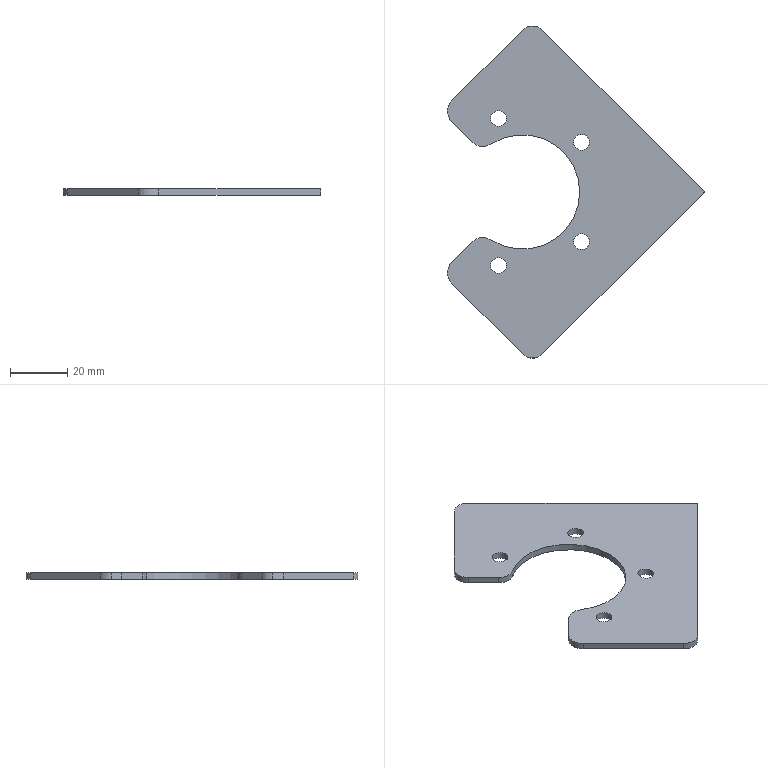Part | SolidWorks | features FlatPattern 1, SMBaseFlange 1, SheetMetal 1 | 1 solid | 25 faces | box 89.853 x 116.066 x 2.3 mm | volume 10484 mm3 | cylinder 17 | plane 8 | commonest cylinder face diameters 5.5 x8 10 x8 40 x1
STEP:
#1=CARTESIAN_POINT('',(-11.093,-25.679,2.3));
#2=VERTEX_POINT('',#1);
#3=CARTESIAN_POINT('',(-5.593,-25.679,2.3));
#4=VERTEX_POINT('',#3);
#5=CARTESIAN_POINT('',(-8.343,-25.679,2.3));
#6=DIRECTION('',(0.,0.,1.));
#7=DIRECTION('',(1.,0.,0.));
#8=AXIS2_PLACEMENT_3D('',#5,#6,#7);
#9=CIRCLE('',#8,2.75);
#10=EDGE_CURVE('',#2,#4,#9,.T.);
#11=ORIENTED_EDGE('',*,*,#10,.T.);
#12=CARTESIAN_POINT('',(-5.593,-25.679,0.));
#13=VERTEX_POINT('',#12);
#14=CARTESIAN_POINT('',(-5.593,-25.679,2.3));
#15=DIRECTION('',(0.,0.,-1.));
#16=VECTOR('',#15,1000.);
#17=LINE('',#14,#16);
#18=EDGE_CURVE('',#4,#13,#17,.T.);
#19=ORIENTED_EDGE('',*,*,#18,.T.);
#20=CARTESIAN_POINT('',(-11.093,-25.679,0.));
#21=VERTEX_POINT('',#20);
#22=CARTESIAN_POINT('',(-8.343,-25.679,0.));
#23=DIRECTION('',(0.,0.,1.));
#24=DIRECTION('',(1.,0.,0.));
#25=AXIS2_PLACEMENT_3D('',#22,#23,#24);
#26=CIRCLE('',#25,2.75);
#27=EDGE_CURVE('',#21,#13,#26,.T.);
#28=ORIENTED_EDGE('',*,*,#27,.F.);
#29=CARTESIAN_POINT('',(-11.093,-25.679,2.3));
#30=DIRECTION('',(0.,0.,-1.));
#31=VECTOR('',#30,1000.);
#32=LINE('',#29,#31);
#33=EDGE_CURVE('',#2,#21,#32,.T.);
#34=ORIENTED_EDGE('',*,*,#33,.F.);
#35=EDGE_LOOP('',(#11,#19,#28,#34));
#36=FACE_OUTER_BOUND('',#35,.T.);
#37=CARTESIAN_POINT('',(-8.343,-25.679,2.3));
#38=DIRECTION('',(0.,0.,-1.));
#39=DIRECTION('',(-1.,0.,0.));
#40=AXIS2_PLACEMENT_3D('',#37,#38,#39);
#41=CYLINDRICAL_SURFACE('',#40,2.75);
#42=ADVANCED_FACE('',(#36),#41,.F.);
#43=CARTESIAN_POINT('',(-11.093,25.679,2.3));
#44=VERTEX_POINT('',#43);
#45=CARTESIAN_POINT('',(-5.593,25.679,2.3));
#46=VERTEX_POINT('',#45);
#47=CARTESIAN_POINT('',(-8.343,25.679,2.3));
#48=DIRECTION('',(0.,0.,1.));
#49=DIRECTION('',(1.,0.,0.));
#50=AXIS2_PLACEMENT_3D('',#47,#48,#49);
#51=CIRCLE('',#50,2.75);
#52=EDGE_CURVE('',#44,#46,#51,.T.);
#53=ORIENTED_EDGE('',*,*,#52,.T.);
#54=CARTESIAN_POINT('',(-5.593,25.679,0.));
#55=VERTEX_POINT('',#54);
#56=CARTESIAN_POINT('',(-5.593,25.679,2.3));
#57=DIRECTION('',(0.,0.,-1.));
#58=VECTOR('',#57,1000.);
#59=LINE('',#56,#58);
#60=EDGE_CURVE('',#46,#55,#59,.T.);
#61=ORIENTED_EDGE('',*,*,#60,.T.);
#62=CARTESIAN_POINT('',(-11.093,25.679,0.));
#63=VERTEX_POINT('',#62);
#64=CARTESIAN_POINT('',(-8.343,25.679,0.));
#65=DIRECTION('',(0.,0.,1.));
#66=DIRECTION('',(1.,0.,0.));
#67=AXIS2_PLACEMENT_3D('',#64,#65,#66);
#68=CIRCLE('',#67,2.75);
#69=EDGE_CURVE('',#63,#55,#68,.T.);
#70=ORIENTED_EDGE('',*,*,#69,.F.);
#71=CARTESIAN_POINT('',(-11.093,25.679,2.3));
#72=DIRECTION('',(0.,0.,-1.));
#73=VECTOR('',#72,1000.);
#74=LINE('',#71,#73);
#75=EDGE_CURVE('',#44,#63,#74,.T.);
#76=ORIENTED_EDGE('',*,*,#75,.F.);
#77=EDGE_LOOP('',(#53,#61,#70,#76));
#78=FACE_OUTER_BOUND('',#77,.T.);
#79=CARTESIAN_POINT('',(-8.343,25.679,2.3));
#80=DIRECTION('',(0.,0.,-1.));
#81=DIRECTION('',(-1.,0.,0.));
#82=AXIS2_PLACEMENT_3D('',#79,#80,#81);
#83=CYLINDRICAL_SURFACE('',#82,2.75);
#84=ADVANCED_FACE('',(#78),#83,.F.);
#85=CARTESIAN_POINT('',(17.933,17.355,2.3));
#86=VERTEX_POINT('',#85);
#87=CARTESIAN_POINT('',(23.433,17.355,2.3));
#88=VERTEX_POINT('',#87);
#89=CARTESIAN_POINT('',(20.683,17.355,2.3));
#90=DIRECTION('',(0.,0.,1.));
#91=DIRECTION('',(1.,0.,0.));
#92=AXIS2_PLACEMENT_3D('',#89,#90,#91);
#93=CIRCLE('',#92,2.75);
#94=EDGE_CURVE('',#86,#88,#93,.T.);
#95=ORIENTED_EDGE('',*,*,#94,.T.);
#96=CARTESIAN_POINT('',(23.433,17.355,0.));
#97=VERTEX_POINT('',#96);
#98=CARTESIAN_POINT('',(23.433,17.355,2.3));
#99=DIRECTION('',(0.,0.,-1.));
#100=VECTOR('',#99,1000.);
#101=LINE('',#98,#100);
#102=EDGE_CURVE('',#88,#97,#101,.T.);
#103=ORIENTED_EDGE('',*,*,#102,.T.);
#104=CARTESIAN_POINT('',(17.933,17.355,0.));
#105=VERTEX_POINT('',#104);
#106=CARTESIAN_POINT('',(20.683,17.355,0.));
#107=DIRECTION('',(0.,0.,1.));
#108=DIRECTION('',(1.,0.,0.));
#109=AXIS2_PLACEMENT_3D('',#106,#107,#108);
#110=CIRCLE('',#109,2.75);
#111=EDGE_CURVE('',#105,#97,#110,.T.);
#112=ORIENTED_EDGE('',*,*,#111,.F.);
#113=CARTESIAN_POINT('',(17.933,17.355,2.3));
#114=DIRECTION('',(0.,0.,-1.));
#115=VECTOR('',#114,1000.);
#116=LINE('',#113,#115);
#117=EDGE_CURVE('',#86,#105,#116,.T.);
#118=ORIENTED_EDGE('',*,*,#117,.F.);
#119=EDGE_LOOP('',(#95,#103,#112,#118));
#120=FACE_OUTER_BOUND('',#119,.T.);
#121=CARTESIAN_POINT('',(20.683,17.355,2.3));
#122=DIRECTION('',(0.,0.,-1.));
#123=DIRECTION('',(-1.,0.,0.));
#124=AXIS2_PLACEMENT_3D('',#121,#122,#123);
#125=CYLINDRICAL_SURFACE('',#124,2.75);
#126=ADVANCED_FACE('',(#120),#125,.F.);
#127=CARTESIAN_POINT('',(17.933,-17.355,2.3));
#128=VERTEX_POINT('',#127);
#129=CARTESIAN_POINT('',(23.433,-17.355,2.3));
#130=VERTEX_POINT('',#129);
#131=CARTESIAN_POINT('',(20.683,-17.355,2.3));
#132=DIRECTION('',(0.,0.,1.));
#133=DIRECTION('',(1.,0.,0.));
#134=AXIS2_PLACEMENT_3D('',#131,#132,#133);
#135=CIRCLE('',#134,2.75);
#136=EDGE_CURVE('',#128,#130,#135,.T.);
#137=ORIENTED_EDGE('',*,*,#136,.T.);
#138=CARTESIAN_POINT('',(23.433,-17.355,0.));
#139=VERTEX_POINT('',#138);
#140=CARTESIAN_POINT('',(23.433,-17.355,2.3));
#141=DIRECTION('',(0.,0.,-1.));
#142=VECTOR('',#141,1000.);
#143=LINE('',#140,#142);
#144=EDGE_CURVE('',#130,#139,#143,.T.);
#145=ORIENTED_EDGE('',*,*,#144,.T.);
#146=CARTESIAN_POINT('',(17.933,-17.355,0.));
#147=VERTEX_POINT('',#146);
#148=CARTESIAN_POINT('',(20.683,-17.355,0.));
#149=DIRECTION('',(0.,0.,1.));
#150=DIRECTION('',(1.,0.,0.));
#151=AXIS2_PLACEMENT_3D('',#148,#149,#150);
#152=CIRCLE('',#151,2.75);
#153=EDGE_CURVE('',#147,#139,#152,.T.);
#154=ORIENTED_EDGE('',*,*,#153,.F.);
#155=CARTESIAN_POINT('',(17.933,-17.355,2.3));
#156=DIRECTION('',(0.,0.,-1.));
#157=VECTOR('',#156,1000.);
#158=LINE('',#155,#157);
#159=EDGE_CURVE('',#128,#147,#158,.T.);
#160=ORIENTED_EDGE('',*,*,#159,.F.);
#161=EDGE_LOOP('',(#137,#145,#154,#160));
#162=FACE_OUTER_BOUND('',#161,.T.);
#163=CARTESIAN_POINT('',(20.683,-17.355,2.3));
#164=DIRECTION('',(0.,0.,-1.));
#165=DIRECTION('',(-1.,0.,0.));
#166=AXIS2_PLACEMENT_3D('',#163,#164,#165);
#167=CYLINDRICAL_SURFACE('',#166,2.75);
#168=ADVANCED_FACE('',(#162),#167,.F.);
#169=CARTESIAN_POINT('',(-26.213,-28.284,2.3));
#170=VERTEX_POINT('',#169);
#171=CARTESIAN_POINT('',(-24.749,-31.82,2.3));
#172=VERTEX_POINT('',#171);
#173=CARTESIAN_POINT('',(-21.213,-28.284,2.3));
#174=DIRECTION('',(0.,0.,1.));
#175=DIRECTION('',(-1.,0.,0.));
#176=AXIS2_PLACEMENT_3D('',#173,#174,#175);
#177=CIRCLE('',#176,5.);
#178=EDGE_CURVE('',#170,#172,#177,.T.);
#179=ORIENTED_EDGE('',*,*,#178,.F.);
#180=CARTESIAN_POINT('',(-26.213,-28.284,0.));
#181=VERTEX_POINT('',#180);
#182=CARTESIAN_POINT('',(-26.213,-28.284,2.3));
#183=DIRECTION('',(0.,0.,-1.));
#184=VECTOR('',#183,1000.);
#185=LINE('',#182,#184);
#186=EDGE_CURVE('',#170,#181,#185,.T.);
#187=ORIENTED_EDGE('',*,*,#186,.T.);
#188=CARTESIAN_POINT('',(-24.749,-31.82,0.));
#189=VERTEX_POINT('',#188);
#190=CARTESIAN_POINT('',(-21.213,-28.284,0.));
#191=DIRECTION('',(0.,0.,1.));
#192=DIRECTION('',(-1.,0.,0.));
#193=AXIS2_PLACEMENT_3D('',#190,#191,#192);
#194=CIRCLE('',#193,5.);
#195=EDGE_CURVE('',#181,#189,#194,.T.);
#196=ORIENTED_EDGE('',*,*,#195,.T.);
#197=CARTESIAN_POINT('',(-24.749,-31.82,2.3));
#198=DIRECTION('',(0.,0.,-1.));
#199=VECTOR('',#198,1000.);
#200=LINE('',#197,#199);
#201=EDGE_CURVE('',#172,#189,#200,.T.);
#202=ORIENTED_EDGE('',*,*,#201,.F.);
#203=EDGE_LOOP('',(#179,#187,#196,#202));
#204=FACE_OUTER_BOUND('',#203,.T.);
#205=CARTESIAN_POINT('',(-21.213,-28.284,2.3));
#206=DIRECTION('',(0.,0.,-1.));
#207=DIRECTION('',(-1.,0.,0.));
#208=AXIS2_PLACEMENT_3D('',#205,#206,#207);
#209=CYLINDRICAL_SURFACE('',#208,5.);
#210=ADVANCED_FACE('',(#204),#209,.T.);
#211=CARTESIAN_POINT('',(-26.213,28.284,2.3));
#212=VERTEX_POINT('',#211);
#213=CARTESIAN_POINT('',(-24.749,24.749,2.3));
#214=VERTEX_POINT('',#213);
#215=CARTESIAN_POINT('',(-21.213,28.284,2.3));
#216=DIRECTION('',(0.,0.,1.));
#217=DIRECTION('',(-1.,0.,0.));
#218=AXIS2_PLACEMENT_3D('',#215,#216,#217);
#219=CIRCLE('',#218,5.);
#220=EDGE_CURVE('',#212,#214,#219,.T.);
#221=ORIENTED_EDGE('',*,*,#220,.F.);
#222=CARTESIAN_POINT('',(-26.213,28.284,0.));
#223=VERTEX_POINT('',#222);
#224=CARTESIAN_POINT('',(-26.213,28.284,2.3));
#225=DIRECTION('',(0.,0.,-1.));
#226=VECTOR('',#225,1000.);
#227=LINE('',#224,#226);
#228=EDGE_CURVE('',#212,#223,#227,.T.);
#229=ORIENTED_EDGE('',*,*,#228,.T.);
#230=CARTESIAN_POINT('',(-24.749,24.749,0.));
#231=VERTEX_POINT('',#230);
#232=CARTESIAN_POINT('',(-21.213,28.284,0.));
#233=DIRECTION('',(0.,0.,1.));
#234=DIRECTION('',(-1.,0.,0.));
#235=AXIS2_PLACEMENT_3D('',#232,#233,#234);
#236=CIRCLE('',#235,5.);
#237=EDGE_CURVE('',#223,#231,#236,.T.);
#238=ORIENTED_EDGE('',*,*,#237,.T.);
#239=CARTESIAN_POINT('',(-24.749,24.749,2.3));
#240=DIRECTION('',(0.,0.,-1.));
#241=VECTOR('',#240,1000.);
#242=LINE('',#239,#241);
#243=EDGE_CURVE('',#214,#231,#242,.T.);
#244=ORIENTED_EDGE('',*,*,#243,.F.);
#245=EDGE_LOOP('',(#221,#229,#238,#244));
#246=FACE_OUTER_BOUND('',#245,.T.);
#247=CARTESIAN_POINT('',(-21.213,28.284,2.3));
#248=DIRECTION('',(0.,0.,-1.));
#249=DIRECTION('',(-1.,0.,0.));
#250=AXIS2_PLACEMENT_3D('',#247,#248,#249);
#251=CYLINDRICAL_SURFACE('',#250,5.);
#252=ADVANCED_FACE('',(#246),#251,.T.);
#253=CARTESIAN_POINT('',(-24.749,31.82,2.3));
#254=VERTEX_POINT('',#253);
#255=CARTESIAN_POINT('',(-21.213,28.284,2.3));
#256=DIRECTION('',(0.,0.,1.));
#257=DIRECTION('',(-1.,0.,0.));
#258=AXIS2_PLACEMENT_3D('',#255,#256,#257);
#259=CIRCLE('',#258,5.);
#260=EDGE_CURVE('',#254,#212,#259,.T.);
#261=ORIENTED_EDGE('',*,*,#260,.T.);
#262=ORIENTED_EDGE('',*,*,#220,.T.);
#263=CARTESIAN_POINT('',(-17.321,17.321,2.3));
#264=VERTEX_POINT('',#263);
#265=CARTESIAN_POINT('',(-17.321,17.321,2.3));
#266=DIRECTION('',(0.7071,-0.7071,0.));
#267=VECTOR('',#266,1000.);
#268=LINE('',#265,#267);
#269=EDGE_CURVE('',#214,#264,#268,.T.);
#270=ORIENTED_EDGE('',*,*,#269,.T.);
#271=CARTESIAN_POINT('',(-11.028,16.685,2.3));
#272=VERTEX_POINT('',#271);
#273=CARTESIAN_POINT('',(-13.785,20.856,2.3));
#274=DIRECTION('',(0.,0.,1.));
#275=DIRECTION('',(1.,0.,0.));
#276=AXIS2_PLACEMENT_3D('',#273,#274,#275);
#277=CIRCLE('',#276,5.);
#278=EDGE_CURVE('',#264,#272,#277,.T.);
#279=ORIENTED_EDGE('',*,*,#278,.T.);
#280=CARTESIAN_POINT('',(-11.028,-16.685,2.3));
#281=VERTEX_POINT('',#280);
#282=CARTESIAN_POINT('',(0.,0.,2.3));
#283=DIRECTION('',(0.,0.,-1.));
#284=DIRECTION('',(1.,0.,0.));
#285=AXIS2_PLACEMENT_3D('',#282,#283,#284);
#286=CIRCLE('',#285,20.);
#287=EDGE_CURVE('',#272,#281,#286,.T.);
#288=ORIENTED_EDGE('',*,*,#287,.T.);
#289=CARTESIAN_POINT('',(-17.321,-17.321,2.3));
#290=VERTEX_POINT('',#289);
#291=CARTESIAN_POINT('',(-13.785,-20.856,2.3));
#292=DIRECTION('',(0.,0.,1.));
#293=DIRECTION('',(-1.,0.,0.));
#294=AXIS2_PLACEMENT_3D('',#291,#292,#293);
#295=CIRCLE('',#294,5.);
#296=EDGE_CURVE('',#281,#290,#295,.T.);
#297=ORIENTED_EDGE('',*,*,#296,.T.);
#298=CARTESIAN_POINT('',(-24.749,-24.749,2.3));
#299=VERTEX_POINT('',#298);
#300=CARTESIAN_POINT('',(-24.749,-24.749,2.3));
#301=DIRECTION('',(-0.7071,-0.7071,0.));
#302=VECTOR('',#301,1000.);
#303=LINE('',#300,#302);
#304=EDGE_CURVE('',#290,#299,#303,.T.);
#305=ORIENTED_EDGE('',*,*,#304,.T.);
#306=CARTESIAN_POINT('',(-21.213,-28.284,2.3));
#307=DIRECTION('',(0.,0.,1.));
#308=DIRECTION('',(-1.,0.,0.));
#309=AXIS2_PLACEMENT_3D('',#306,#307,#308);
#310=CIRCLE('',#309,5.);
#311=EDGE_CURVE('',#299,#170,#310,.T.);
#312=ORIENTED_EDGE('',*,*,#311,.T.);
#313=ORIENTED_EDGE('',*,*,#178,.T.);
#314=CARTESIAN_POINT('',(0.00006304,-56.568,2.3));
#315=VERTEX_POINT('',#314);
#316=CARTESIAN_POINT('',(0.00006304,-56.568,2.3));
#317=DIRECTION('',(0.7071,-0.7071,0.));
#318=VECTOR('',#317,1000.);
#319=LINE('',#316,#318);
#320=EDGE_CURVE('',#172,#315,#319,.T.);
#321=ORIENTED_EDGE('',*,*,#320,.T.);
#322=CARTESIAN_POINT('',(7.071,-56.568,2.3));
#323=VERTEX_POINT('',#322);
#324=CARTESIAN_POINT('',(3.536,-53.033,2.3));
#325=DIRECTION('',(0.,0.,1.));
#326=DIRECTION('',(1.,0.,0.));
#327=AXIS2_PLACEMENT_3D('',#324,#325,#326);
#328=CIRCLE('',#327,5.);
#329=EDGE_CURVE('',#315,#323,#328,.T.);
#330=ORIENTED_EDGE('',*,*,#329,.T.);
#331=CARTESIAN_POINT('',(63.64,0.00006304,2.3));
#332=VERTEX_POINT('',#331);
#333=CARTESIAN_POINT('',(7.071,-56.568,2.3));
#334=DIRECTION('',(0.7071,0.7071,0.));
#335=VECTOR('',#334,1000.);
#336=LINE('',#333,#335);
#337=EDGE_CURVE('',#323,#332,#336,.T.);
#338=ORIENTED_EDGE('',*,*,#337,.T.);
#339=CARTESIAN_POINT('',(7.071,56.569,2.3));
#340=VERTEX_POINT('',#339);
#341=CARTESIAN_POINT('',(7.071,56.569,2.3));
#342=DIRECTION('',(-0.7071,0.7071,0.));
#343=VECTOR('',#342,1000.);
#344=LINE('',#341,#343);
#345=EDGE_CURVE('',#332,#340,#344,.T.);
#346=ORIENTED_EDGE('',*,*,#345,.T.);
#347=CARTESIAN_POINT('',(0.000003708,56.569,2.3));
#348=VERTEX_POINT('',#347);
#349=CARTESIAN_POINT('',(3.536,53.033,2.3));
#350=DIRECTION('',(0.,0.,1.));
#351=DIRECTION('',(-1.,0.,0.));
#352=AXIS2_PLACEMENT_3D('',#349,#350,#351);
#353=CIRCLE('',#352,5.);
#354=EDGE_CURVE('',#340,#348,#353,.T.);
#355=ORIENTED_EDGE('',*,*,#354,.T.);
#356=CARTESIAN_POINT('',(-24.749,31.82,2.3));
#357=DIRECTION('',(-0.7071,-0.7071,0.));
#358=VECTOR('',#357,1000.);
#359=LINE('',#356,#358);
#360=EDGE_CURVE('',#348,#254,#359,.T.);
#361=ORIENTED_EDGE('',*,*,#360,.T.);
#362=EDGE_LOOP('',(#261,#262,#270,#279,#288,#297,#305,#312,#313,#321,#330,#338,#346,#355,#361));
#363=FACE_OUTER_BOUND('',#362,.T.);
#364=ORIENTED_EDGE('',*,*,#136,.F.);
#365=CARTESIAN_POINT('',(20.683,-17.355,2.3));
#366=DIRECTION('',(0.,0.,1.));
#367=DIRECTION('',(1.,0.,0.));
#368=AXIS2_PLACEMENT_3D('',#365,#366,#367);
#369=CIRCLE('',#368,2.75);
#370=EDGE_CURVE('',#130,#128,#369,.T.);
#371=ORIENTED_EDGE('',*,*,#370,.F.);
#372=EDGE_LOOP('',(#364,#371));
#373=FACE_BOUND('',#372,.T.);
#374=ORIENTED_EDGE('',*,*,#94,.F.);
#375=CARTESIAN_POINT('',(20.683,17.355,2.3));
#376=DIRECTION('',(0.,0.,1.));
#377=DIRECTION('',(1.,0.,0.));
#378=AXIS2_PLACEMENT_3D('',#375,#376,#377);
#379=CIRCLE('',#378,2.75);
#380=EDGE_CURVE('',#88,#86,#379,.T.);
#381=ORIENTED_EDGE('',*,*,#380,.F.);
#382=EDGE_LOOP('',(#374,#381));
#383=FACE_BOUND('',#382,.T.);
#384=ORIENTED_EDGE('',*,*,#52,.F.);
#385=CARTESIAN_POINT('',(-8.343,25.679,2.3));
#386=DIRECTION('',(0.,0.,1.));
#387=DIRECTION('',(1.,0.,0.));
#388=AXIS2_PLACEMENT_3D('',#385,#386,#387);
#389=CIRCLE('',#388,2.75);
#390=EDGE_CURVE('',#46,#44,#389,.T.);
#391=ORIENTED_EDGE('',*,*,#390,.F.);
#392=EDGE_LOOP('',(#384,#391));
#393=FACE_BOUND('',#392,.T.);
#394=ORIENTED_EDGE('',*,*,#10,.F.);
#395=CARTESIAN_POINT('',(-8.343,-25.679,2.3));
#396=DIRECTION('',(0.,0.,1.));
#397=DIRECTION('',(1.,0.,0.));
#398=AXIS2_PLACEMENT_3D('',#395,#396,#397);
#399=CIRCLE('',#398,2.75);
#400=EDGE_CURVE('',#4,#2,#399,.T.);
#401=ORIENTED_EDGE('',*,*,#400,.F.);
#402=EDGE_LOOP('',(#394,#401));
#403=FACE_BOUND('',#402,.T.);
#404=CARTESIAN_POINT('',(-21.213,28.284,2.3));
#405=DIRECTION('',(0.,0.,-1.));
#406=DIRECTION('',(-1.,0.,0.));
#407=AXIS2_PLACEMENT_3D('',#404,#405,#406);
#408=PLANE('',#407);
#409=ADVANCED_FACE('',(#363,#373,#383,#393,#403),#408,.F.);
#410=ORIENTED_EDGE('',*,*,#69,.T.);
#411=CARTESIAN_POINT('',(-8.343,25.679,0.));
#412=DIRECTION('',(0.,0.,1.));
#413=DIRECTION('',(1.,0.,0.));
#414=AXIS2_PLACEMENT_3D('',#411,#412,#413);
#415=CIRCLE('',#414,2.75);
#416=EDGE_CURVE('',#55,#63,#415,.T.);
#417=ORIENTED_EDGE('',*,*,#416,.T.);
#418=EDGE_LOOP('',(#410,#417));
#419=FACE_BOUND('',#418,.T.);
#420=ORIENTED_EDGE('',*,*,#153,.T.);
#421=CARTESIAN_POINT('',(20.683,-17.355,0.));
#422=DIRECTION('',(0.,0.,1.));
#423=DIRECTION('',(1.,0.,0.));
#424=AXIS2_PLACEMENT_3D('',#421,#422,#423);
#425=CIRCLE('',#424,2.75);
#426=EDGE_CURVE('',#139,#147,#425,.T.);
#427=ORIENTED_EDGE('',*,*,#426,.T.);
#428=EDGE_LOOP('',(#420,#427));
#429=FACE_BOUND('',#428,.T.);
#430=CARTESIAN_POINT('',(-24.749,31.82,0.));
#431=VERTEX_POINT('',#430);
#432=CARTESIAN_POINT('',(-21.213,28.284,0.));
#433=DIRECTION('',(0.,0.,1.));
#434=DIRECTION('',(-1.,0.,0.));
#435=AXIS2_PLACEMENT_3D('',#432,#433,#434);
#436=CIRCLE('',#435,5.);
#437=EDGE_CURVE('',#431,#223,#436,.T.);
#438=ORIENTED_EDGE('',*,*,#437,.F.);
#439=CARTESIAN_POINT('',(0.000003708,56.569,0.));
#440=VERTEX_POINT('',#439);
#441=CARTESIAN_POINT('',(-24.749,31.82,0.));
#442=DIRECTION('',(-0.7071,-0.7071,0.));
#443=VECTOR('',#442,1000.);
#444=LINE('',#441,#443);
#445=EDGE_CURVE('',#440,#431,#444,.T.);
#446=ORIENTED_EDGE('',*,*,#445,.F.);
#447=CARTESIAN_POINT('',(7.071,56.569,0.));
#448=VERTEX_POINT('',#447);
#449=CARTESIAN_POINT('',(3.536,53.033,0.));
#450=DIRECTION('',(0.,0.,1.));
#451=DIRECTION('',(-1.,0.,0.));
#452=AXIS2_PLACEMENT_3D('',#449,#450,#451);
#453=CIRCLE('',#452,5.);
#454=EDGE_CURVE('',#448,#440,#453,.T.);
#455=ORIENTED_EDGE('',*,*,#454,.F.);
#456=CARTESIAN_POINT('',(63.64,0.00006304,0.));
#457=VERTEX_POINT('',#456);
#458=CARTESIAN_POINT('',(7.071,56.569,0.));
#459=DIRECTION('',(-0.7071,0.7071,0.));
#460=VECTOR('',#459,1000.);
#461=LINE('',#458,#460);
#462=EDGE_CURVE('',#457,#448,#461,.T.);
#463=ORIENTED_EDGE('',*,*,#462,.F.);
#464=CARTESIAN_POINT('',(7.071,-56.568,0.));
#465=VERTEX_POINT('',#464);
#466=CARTESIAN_POINT('',(7.071,-56.568,0.));
#467=DIRECTION('',(0.7071,0.7071,0.));
#468=VECTOR('',#467,1000.);
#469=LINE('',#466,#468);
#470=EDGE_CURVE('',#465,#457,#469,.T.);
#471=ORIENTED_EDGE('',*,*,#470,.F.);
#472=CARTESIAN_POINT('',(0.00006304,-56.568,0.));
#473=VERTEX_POINT('',#472);
#474=CARTESIAN_POINT('',(3.536,-53.033,0.));
#475=DIRECTION('',(0.,0.,1.));
#476=DIRECTION('',(1.,0.,0.));
#477=AXIS2_PLACEMENT_3D('',#474,#475,#476);
#478=CIRCLE('',#477,5.);
#479=EDGE_CURVE('',#473,#465,#478,.T.);
#480=ORIENTED_EDGE('',*,*,#479,.F.);
#481=CARTESIAN_POINT('',(0.00006304,-56.568,0.));
#482=DIRECTION('',(0.7071,-0.7071,0.));
#483=VECTOR('',#482,1000.);
#484=LINE('',#481,#483);
#485=EDGE_CURVE('',#189,#473,#484,.T.);
#486=ORIENTED_EDGE('',*,*,#485,.F.);
#487=ORIENTED_EDGE('',*,*,#195,.F.);
#488=CARTESIAN_POINT('',(-24.749,-24.749,0.));
#489=VERTEX_POINT('',#488);
#490=CARTESIAN_POINT('',(-21.213,-28.284,0.));
#491=DIRECTION('',(0.,0.,1.));
#492=DIRECTION('',(-1.,0.,0.));
#493=AXIS2_PLACEMENT_3D('',#490,#491,#492);
#494=CIRCLE('',#493,5.);
#495=EDGE_CURVE('',#489,#181,#494,.T.);
#496=ORIENTED_EDGE('',*,*,#495,.F.);
#497=CARTESIAN_POINT('',(-17.321,-17.321,0.));
#498=VERTEX_POINT('',#497);
#499=CARTESIAN_POINT('',(-24.749,-24.749,0.));
#500=DIRECTION('',(-0.7071,-0.7071,0.));
#501=VECTOR('',#500,1000.);
#502=LINE('',#499,#501);
#503=EDGE_CURVE('',#498,#489,#502,.T.);
#504=ORIENTED_EDGE('',*,*,#503,.F.);
#505=CARTESIAN_POINT('',(-11.028,-16.685,0.));
#506=VERTEX_POINT('',#505);
#507=CARTESIAN_POINT('',(-13.785,-20.856,0.));
#508=DIRECTION('',(0.,0.,1.));
#509=DIRECTION('',(-1.,0.,0.));
#510=AXIS2_PLACEMENT_3D('',#507,#508,#509);
#511=CIRCLE('',#510,5.);
#512=EDGE_CURVE('',#506,#498,#511,.T.);
#513=ORIENTED_EDGE('',*,*,#512,.F.);
#514=CARTESIAN_POINT('',(-11.028,16.685,0.));
#515=VERTEX_POINT('',#514);
#516=CARTESIAN_POINT('',(0.,0.,0.));
#517=DIRECTION('',(0.,0.,-1.));
#518=DIRECTION('',(1.,0.,0.));
#519=AXIS2_PLACEMENT_3D('',#516,#517,#518);
#520=CIRCLE('',#519,20.);
#521=EDGE_CURVE('',#515,#506,#520,.T.);
#522=ORIENTED_EDGE('',*,*,#521,.F.);
#523=CARTESIAN_POINT('',(-17.321,17.321,0.));
#524=VERTEX_POINT('',#523);
#525=CARTESIAN_POINT('',(-13.785,20.856,0.));
#526=DIRECTION('',(0.,0.,1.));
#527=DIRECTION('',(1.,0.,0.));
#528=AXIS2_PLACEMENT_3D('',#525,#526,#527);
#529=CIRCLE('',#528,5.);
#530=EDGE_CURVE('',#524,#515,#529,.T.);
#531=ORIENTED_EDGE('',*,*,#530,.F.);
#532=CARTESIAN_POINT('',(-17.321,17.321,0.));
#533=DIRECTION('',(0.7071,-0.7071,0.));
#534=VECTOR('',#533,1000.);
#535=LINE('',#532,#534);
#536=EDGE_CURVE('',#231,#524,#535,.T.);
#537=ORIENTED_EDGE('',*,*,#536,.F.);
#538=ORIENTED_EDGE('',*,*,#237,.F.);
#539=EDGE_LOOP('',(#438,#446,#455,#463,#471,#480,#486,#487,#496,#504,#513,#522,#531,#537,#538));
#540=FACE_OUTER_BOUND('',#539,.T.);
#541=ORIENTED_EDGE('',*,*,#111,.T.);
#542=CARTESIAN_POINT('',(20.683,17.355,0.));
#543=DIRECTION('',(0.,0.,1.));
#544=DIRECTION('',(1.,0.,0.));
#545=AXIS2_PLACEMENT_3D('',#542,#543,#544);
#546=CIRCLE('',#545,2.75);
#547=EDGE_CURVE('',#97,#105,#546,.T.);
#548=ORIENTED_EDGE('',*,*,#547,.T.);
#549=EDGE_LOOP('',(#541,#548));
#550=FACE_BOUND('',#549,.T.);
#551=ORIENTED_EDGE('',*,*,#27,.T.);
#552=CARTESIAN_POINT('',(-8.343,-25.679,0.));
#553=DIRECTION('',(0.,0.,1.));
#554=DIRECTION('',(1.,0.,0.));
#555=AXIS2_PLACEMENT_3D('',#552,#553,#554);
#556=CIRCLE('',#555,2.75);
#557=EDGE_CURVE('',#13,#21,#556,.T.);
#558=ORIENTED_EDGE('',*,*,#557,.T.);
#559=EDGE_LOOP('',(#551,#558));
#560=FACE_BOUND('',#559,.T.);
#561=CARTESIAN_POINT('',(-21.213,28.284,0.));
#562=DIRECTION('',(0.,0.,-1.));
#563=DIRECTION('',(-1.,0.,0.));
#564=AXIS2_PLACEMENT_3D('',#561,#562,#563);
#565=PLANE('',#564);
#566=ADVANCED_FACE('',(#419,#429,#540,#550,#560),#565,.T.);
#567=ORIENTED_EDGE('',*,*,#228,.F.);
#568=ORIENTED_EDGE('',*,*,#260,.F.);
#569=CARTESIAN_POINT('',(-24.749,31.82,2.3));
#570=DIRECTION('',(0.,0.,-1.));
#571=VECTOR('',#570,1000.);
#572=LINE('',#569,#571);
#573=EDGE_CURVE('',#254,#431,#572,.T.);
#574=ORIENTED_EDGE('',*,*,#573,.T.);
#575=ORIENTED_EDGE('',*,*,#437,.T.);
#576=EDGE_LOOP('',(#567,#568,#574,#575));
#577=FACE_OUTER_BOUND('',#576,.T.);
#578=CARTESIAN_POINT('',(-21.213,28.284,2.3));
#579=DIRECTION('',(0.,0.,-1.));
#580=DIRECTION('',(-1.,0.,0.));
#581=AXIS2_PLACEMENT_3D('',#578,#579,#580);
#582=CYLINDRICAL_SURFACE('',#581,5.);
#583=ADVANCED_FACE('',(#577),#582,.T.);
#584=ORIENTED_EDGE('',*,*,#536,.T.);
#585=CARTESIAN_POINT('',(-17.321,17.321,2.3));
#586=DIRECTION('',(0.,0.,-1.));
#587=VECTOR('',#586,1000.);
#588=LINE('',#585,#587);
#589=EDGE_CURVE('',#264,#524,#588,.T.);
#590=ORIENTED_EDGE('',*,*,#589,.F.);
#591=ORIENTED_EDGE('',*,*,#269,.F.);
#592=ORIENTED_EDGE('',*,*,#243,.T.);
#593=EDGE_LOOP('',(#584,#590,#591,#592));
#594=FACE_OUTER_BOUND('',#593,.T.);
#595=CARTESIAN_POINT('',(-17.321,17.321,2.3));
#596=DIRECTION('',(0.7071,0.7071,0.));
#597=DIRECTION('',(-0.7071,0.7071,0.));
#598=AXIS2_PLACEMENT_3D('',#595,#596,#597);
#599=PLANE('',#598);
#600=ADVANCED_FACE('',(#594),#599,.F.);
#601=ORIENTED_EDGE('',*,*,#530,.T.);
#602=CARTESIAN_POINT('',(-11.028,16.685,2.3));
#603=DIRECTION('',(0.,0.,-1.));
#604=VECTOR('',#603,1000.);
#605=LINE('',#602,#604);
#606=EDGE_CURVE('',#272,#515,#605,.T.);
#607=ORIENTED_EDGE('',*,*,#606,.F.);
#608=ORIENTED_EDGE('',*,*,#278,.F.);
#609=ORIENTED_EDGE('',*,*,#589,.T.);
#610=EDGE_LOOP('',(#601,#607,#608,#609));
#611=FACE_OUTER_BOUND('',#610,.T.);
#612=CARTESIAN_POINT('',(-13.785,20.856,2.3));
#613=DIRECTION('',(0.,0.,-1.));
#614=DIRECTION('',(-1.,0.,0.));
#615=AXIS2_PLACEMENT_3D('',#612,#613,#614);
#616=CYLINDRICAL_SURFACE('',#615,5.);
#617=ADVANCED_FACE('',(#611),#616,.T.);
#618=ORIENTED_EDGE('',*,*,#521,.T.);
#619=CARTESIAN_POINT('',(-11.028,-16.685,2.3));
#620=DIRECTION('',(0.,0.,-1.));
#621=VECTOR('',#620,1000.);
#622=LINE('',#619,#621);
#623=EDGE_CURVE('',#281,#506,#622,.T.);
#624=ORIENTED_EDGE('',*,*,#623,.F.);
#625=ORIENTED_EDGE('',*,*,#287,.F.);
#626=ORIENTED_EDGE('',*,*,#606,.T.);
#627=EDGE_LOOP('',(#618,#624,#625,#626));
#628=FACE_OUTER_BOUND('',#627,.T.);
#629=CARTESIAN_POINT('',(0.,0.,2.3));
#630=DIRECTION('',(0.,0.,-1.));
#631=DIRECTION('',(-1.,0.,0.));
#632=AXIS2_PLACEMENT_3D('',#629,#630,#631);
#633=CYLINDRICAL_SURFACE('',#632,20.);
#634=ADVANCED_FACE('',(#628),#633,.F.);
#635=ORIENTED_EDGE('',*,*,#512,.T.);
#636=CARTESIAN_POINT('',(-17.321,-17.321,2.3));
#637=DIRECTION('',(0.,0.,-1.));
#638=VECTOR('',#637,1000.);
#639=LINE('',#636,#638);
#640=EDGE_CURVE('',#290,#498,#639,.T.);
#641=ORIENTED_EDGE('',*,*,#640,.F.);
#642=ORIENTED_EDGE('',*,*,#296,.F.);
#643=ORIENTED_EDGE('',*,*,#623,.T.);
#644=EDGE_LOOP('',(#635,#641,#642,#643));
#645=FACE_OUTER_BOUND('',#644,.T.);
#646=CARTESIAN_POINT('',(-13.785,-20.856,2.3));
#647=DIRECTION('',(0.,0.,-1.));
#648=DIRECTION('',(-1.,0.,0.));
#649=AXIS2_PLACEMENT_3D('',#646,#647,#648);
#650=CYLINDRICAL_SURFACE('',#649,5.);
#651=ADVANCED_FACE('',(#645),#650,.T.);
#652=ORIENTED_EDGE('',*,*,#503,.T.);
#653=CARTESIAN_POINT('',(-24.749,-24.749,2.3));
#654=DIRECTION('',(0.,0.,-1.));
#655=VECTOR('',#654,1000.);
#656=LINE('',#653,#655);
#657=EDGE_CURVE('',#299,#489,#656,.T.);
#658=ORIENTED_EDGE('',*,*,#657,.F.);
#659=ORIENTED_EDGE('',*,*,#304,.F.);
#660=ORIENTED_EDGE('',*,*,#640,.T.);
#661=EDGE_LOOP('',(#652,#658,#659,#660));
#662=FACE_OUTER_BOUND('',#661,.T.);
#663=CARTESIAN_POINT('',(-24.749,-24.749,2.3));
#664=DIRECTION('',(0.7071,-0.7071,0.));
#665=DIRECTION('',(0.7071,0.7071,0.));
#666=AXIS2_PLACEMENT_3D('',#663,#664,#665);
#667=PLANE('',#666);
#668=ADVANCED_FACE('',(#662),#667,.F.);
#669=ORIENTED_EDGE('',*,*,#186,.F.);
#670=ORIENTED_EDGE('',*,*,#311,.F.);
#671=ORIENTED_EDGE('',*,*,#657,.T.);
#672=ORIENTED_EDGE('',*,*,#495,.T.);
#673=EDGE_LOOP('',(#669,#670,#671,#672));
#674=FACE_OUTER_BOUND('',#673,.T.);
#675=CARTESIAN_POINT('',(-21.213,-28.284,2.3));
#676=DIRECTION('',(0.,0.,-1.));
#677=DIRECTION('',(-1.,0.,0.));
#678=AXIS2_PLACEMENT_3D('',#675,#676,#677);
#679=CYLINDRICAL_SURFACE('',#678,5.);
#680=ADVANCED_FACE('',(#674),#679,.T.);
#681=ORIENTED_EDGE('',*,*,#485,.T.);
#682=CARTESIAN_POINT('',(0.00006304,-56.568,2.3));
#683=DIRECTION('',(0.,0.,-1.));
#684=VECTOR('',#683,1000.);
#685=LINE('',#682,#684);
#686=EDGE_CURVE('',#315,#473,#685,.T.);
#687=ORIENTED_EDGE('',*,*,#686,.F.);
#688=ORIENTED_EDGE('',*,*,#320,.F.);
#689=ORIENTED_EDGE('',*,*,#201,.T.);
#690=EDGE_LOOP('',(#681,#687,#688,#689));
#691=FACE_OUTER_BOUND('',#690,.T.);
#692=CARTESIAN_POINT('',(0.00006304,-56.568,2.3));
#693=DIRECTION('',(0.7071,0.7071,0.));
#694=DIRECTION('',(-0.7071,0.7071,0.));
#695=AXIS2_PLACEMENT_3D('',#692,#693,#694);
#696=PLANE('',#695);
#697=ADVANCED_FACE('',(#691),#696,.F.);
#698=ORIENTED_EDGE('',*,*,#479,.T.);
#699=CARTESIAN_POINT('',(7.071,-56.568,2.3));
#700=DIRECTION('',(0.,0.,-1.));
#701=VECTOR('',#700,1000.);
#702=LINE('',#699,#701);
#703=EDGE_CURVE('',#323,#465,#702,.T.);
#704=ORIENTED_EDGE('',*,*,#703,.F.);
#705=ORIENTED_EDGE('',*,*,#329,.F.);
#706=ORIENTED_EDGE('',*,*,#686,.T.);
#707=EDGE_LOOP('',(#698,#704,#705,#706));
#708=FACE_OUTER_BOUND('',#707,.T.);
#709=CARTESIAN_POINT('',(3.536,-53.033,2.3));
#710=DIRECTION('',(0.,0.,-1.));
#711=DIRECTION('',(-1.,0.,0.));
#712=AXIS2_PLACEMENT_3D('',#709,#710,#711);
#713=CYLINDRICAL_SURFACE('',#712,5.);
#714=ADVANCED_FACE('',(#708),#713,.T.);
#715=ORIENTED_EDGE('',*,*,#470,.T.);
#716=CARTESIAN_POINT('',(63.64,0.00006304,2.3));
#717=DIRECTION('',(0.,0.,-1.));
#718=VECTOR('',#717,1000.);
#719=LINE('',#716,#718);
#720=EDGE_CURVE('',#332,#457,#719,.T.);
#721=ORIENTED_EDGE('',*,*,#720,.F.);
#722=ORIENTED_EDGE('',*,*,#337,.F.);
#723=ORIENTED_EDGE('',*,*,#703,.T.);
#724=EDGE_LOOP('',(#715,#721,#722,#723));
#725=FACE_OUTER_BOUND('',#724,.T.);
#726=CARTESIAN_POINT('',(7.071,-56.568,2.3));
#727=DIRECTION('',(-0.7071,0.7071,0.));
#728=DIRECTION('',(-0.7071,-0.7071,0.));
#729=AXIS2_PLACEMENT_3D('',#726,#727,#728);
#730=PLANE('',#729);
#731=ADVANCED_FACE('',(#725),#730,.F.);
#732=ORIENTED_EDGE('',*,*,#462,.T.);
#733=CARTESIAN_POINT('',(7.071,56.569,2.3));
#734=DIRECTION('',(0.,0.,-1.));
#735=VECTOR('',#734,1000.);
#736=LINE('',#733,#735);
#737=EDGE_CURVE('',#340,#448,#736,.T.);
#738=ORIENTED_EDGE('',*,*,#737,.F.);
#739=ORIENTED_EDGE('',*,*,#345,.F.);
#740=ORIENTED_EDGE('',*,*,#720,.T.);
#741=EDGE_LOOP('',(#732,#738,#739,#740));
#742=FACE_OUTER_BOUND('',#741,.T.);
#743=CARTESIAN_POINT('',(7.071,56.569,2.3));
#744=DIRECTION('',(-0.7071,-0.7071,0.));
#745=DIRECTION('',(0.7071,-0.7071,0.));
#746=AXIS2_PLACEMENT_3D('',#743,#744,#745);
#747=PLANE('',#746);
#748=ADVANCED_FACE('',(#742),#747,.F.);
#749=ORIENTED_EDGE('',*,*,#454,.T.);
#750=CARTESIAN_POINT('',(0.000003708,56.569,2.3));
#751=DIRECTION('',(0.,0.,-1.));
#752=VECTOR('',#751,1000.);
#753=LINE('',#750,#752);
#754=EDGE_CURVE('',#348,#440,#753,.T.);
#755=ORIENTED_EDGE('',*,*,#754,.F.);
#756=ORIENTED_EDGE('',*,*,#354,.F.);
#757=ORIENTED_EDGE('',*,*,#737,.T.);
#758=EDGE_LOOP('',(#749,#755,#756,#757));
#759=FACE_OUTER_BOUND('',#758,.T.);
#760=CARTESIAN_POINT('',(3.536,53.033,2.3));
#761=DIRECTION('',(0.,0.,-1.));
#762=DIRECTION('',(-1.,0.,0.));
#763=AXIS2_PLACEMENT_3D('',#760,#761,#762);
#764=CYLINDRICAL_SURFACE('',#763,5.);
#765=ADVANCED_FACE('',(#759),#764,.T.);
#766=ORIENTED_EDGE('',*,*,#445,.T.);
#767=ORIENTED_EDGE('',*,*,#573,.F.);
#768=ORIENTED_EDGE('',*,*,#360,.F.);
#769=ORIENTED_EDGE('',*,*,#754,.T.);
#770=EDGE_LOOP('',(#766,#767,#768,#769));
#771=FACE_OUTER_BOUND('',#770,.T.);
#772=CARTESIAN_POINT('',(-24.749,31.82,2.3));
#773=DIRECTION('',(0.7071,-0.7071,0.));
#774=DIRECTION('',(0.7071,0.7071,0.));
#775=AXIS2_PLACEMENT_3D('',#772,#773,#774);
#776=PLANE('',#775);
#777=ADVANCED_FACE('',(#771),#776,.F.);
#778=ORIENTED_EDGE('',*,*,#144,.F.);
#779=ORIENTED_EDGE('',*,*,#370,.T.);
#780=ORIENTED_EDGE('',*,*,#159,.T.);
#781=ORIENTED_EDGE('',*,*,#426,.F.);
#782=EDGE_LOOP('',(#778,#779,#780,#781));
#783=FACE_OUTER_BOUND('',#782,.T.);
#784=CARTESIAN_POINT('',(20.683,-17.355,2.3));
#785=DIRECTION('',(0.,0.,-1.));
#786=DIRECTION('',(-1.,0.,0.));
#787=AXIS2_PLACEMENT_3D('',#784,#785,#786);
#788=CYLINDRICAL_SURFACE('',#787,2.75);
#789=ADVANCED_FACE('',(#783),#788,.F.);
#790=ORIENTED_EDGE('',*,*,#102,.F.);
#791=ORIENTED_EDGE('',*,*,#380,.T.);
#792=ORIENTED_EDGE('',*,*,#117,.T.);
#793=ORIENTED_EDGE('',*,*,#547,.F.);
#794=EDGE_LOOP('',(#790,#791,#792,#793));
#795=FACE_OUTER_BOUND('',#794,.T.);
#796=CARTESIAN_POINT('',(20.683,17.355,2.3));
#797=DIRECTION('',(0.,0.,-1.));
#798=DIRECTION('',(-1.,0.,0.));
#799=AXIS2_PLACEMENT_3D('',#796,#797,#798);
#800=CYLINDRICAL_SURFACE('',#799,2.75);
#801=ADVANCED_FACE('',(#795),#800,.F.);
#802=ORIENTED_EDGE('',*,*,#60,.F.);
#803=ORIENTED_EDGE('',*,*,#390,.T.);
#804=ORIENTED_EDGE('',*,*,#75,.T.);
#805=ORIENTED_EDGE('',*,*,#416,.F.);
#806=EDGE_LOOP('',(#802,#803,#804,#805));
#807=FACE_OUTER_BOUND('',#806,.T.);
#808=CARTESIAN_POINT('',(-8.343,25.679,2.3));
#809=DIRECTION('',(0.,0.,-1.));
#810=DIRECTION('',(-1.,0.,0.));
#811=AXIS2_PLACEMENT_3D('',#808,#809,#810);
#812=CYLINDRICAL_SURFACE('',#811,2.75);
#813=ADVANCED_FACE('',(#807),#812,.F.);
#814=ORIENTED_EDGE('',*,*,#18,.F.);
#815=ORIENTED_EDGE('',*,*,#400,.T.);
#816=ORIENTED_EDGE('',*,*,#33,.T.);
#817=ORIENTED_EDGE('',*,*,#557,.F.);
#818=EDGE_LOOP('',(#814,#815,#816,#817));
#819=FACE_OUTER_BOUND('',#818,.T.);
#820=CARTESIAN_POINT('',(-8.343,-25.679,2.3));
#821=DIRECTION('',(0.,0.,-1.));
#822=DIRECTION('',(-1.,0.,0.));
#823=AXIS2_PLACEMENT_3D('',#820,#821,#822);
#824=CYLINDRICAL_SURFACE('',#823,2.75);
#825=ADVANCED_FACE('',(#819),#824,.F.);
#826=CLOSED_SHELL('',(#42,#84,#126,#168,#210,#252,#409,#566,#583,#600,#617,#634,#651,#668,#680,#697,#714,#731,#748,#765,#777,#789,#801,#813,#825));
#827=MANIFOLD_SOLID_BREP('',#826);
#828=CARTESIAN_POINT('',(0.,0.,0.));
#829=DIRECTION('',(0.,0.,1.));
#830=DIRECTION('',(1.,0.,0.));
#831=AXIS2_PLACEMENT_3D('',#828,#829,#830);
#832=(LENGTH_UNIT()NAMED_UNIT(*)SI_UNIT(.MILLI.,.METRE.));
#833=UNCERTAINTY_MEASURE_WITH_UNIT(LENGTH_MEASURE(0.00001),#832,'','');
#834=(NAMED_UNIT(*)PLANE_ANGLE_UNIT()SI_UNIT($,.RADIAN.));
#835=(NAMED_UNIT(*)SI_UNIT($,.STERADIAN.)SOLID_ANGLE_UNIT());
#836=(GEOMETRIC_REPRESENTATION_CONTEXT(3)GLOBAL_UNCERTAINTY_ASSIGNED_CONTEXT((#833))GLOBAL_UNIT_ASSIGNED_CONTEXT((#832,#834,#835))REPRESENTATION_CONTEXT('',''));
#837=ADVANCED_BREP_SHAPE_REPRESENTATION('',(#827,#831),#836);